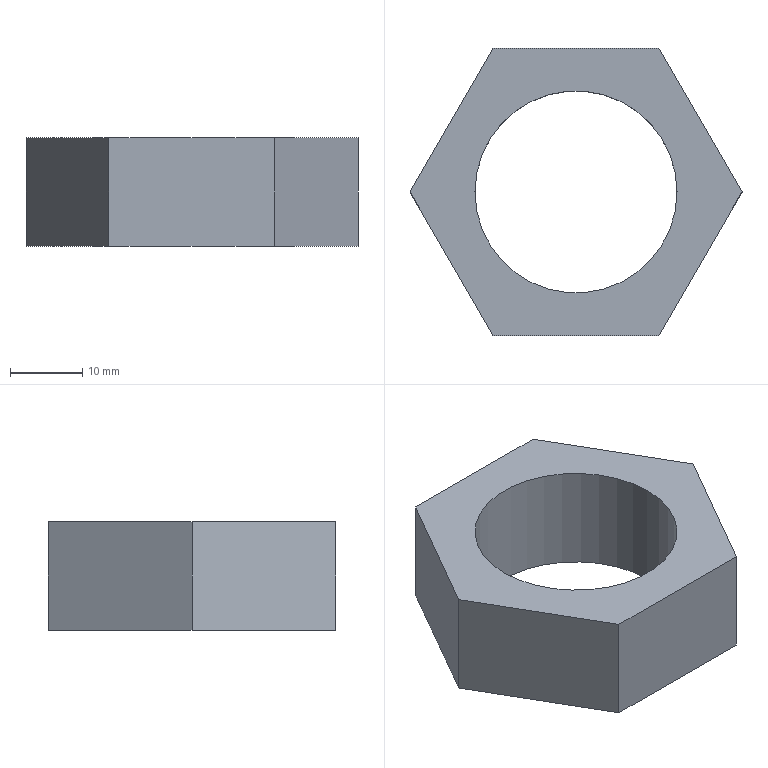Part | NX | features solid 2 | 1 solid | 9 faces | box 46 x 39.837 x 15 mm | volume 11379 mm3 | plane 8 | cylinder 1 | commonest cylinder face diameters 28 x1
STEP:
#1=CARTESIAN_POINT('',(11.5,-174.919,-70.));
#2=VERTEX_POINT('',#1);
#3=CARTESIAN_POINT('',(-11.5,-174.919,-70.));
#4=VERTEX_POINT('',#3);
#5=CARTESIAN_POINT('',(11.5,-174.919,-70.));
#6=DIRECTION('',(-1.,0.,0.));
#7=VECTOR('',#6,1000.);
#8=LINE('',#5,#7);
#9=EDGE_CURVE('',#2,#4,#8,.T.);
#10=ORIENTED_EDGE('',*,*,#9,.F.);
#11=CARTESIAN_POINT('',(11.5,-174.919,-55.));
#12=VERTEX_POINT('',#11);
#13=CARTESIAN_POINT('',(11.5,-174.919,-55.));
#14=DIRECTION('',(0.,0.,-1.));
#15=VECTOR('',#14,1000.);
#16=LINE('',#13,#15);
#17=EDGE_CURVE('',#12,#2,#16,.T.);
#18=ORIENTED_EDGE('',*,*,#17,.F.);
#19=CARTESIAN_POINT('',(-11.5,-174.919,-55.));
#20=VERTEX_POINT('',#19);
#21=CARTESIAN_POINT('',(11.5,-174.919,-55.));
#22=DIRECTION('',(-1.,0.,0.));
#23=VECTOR('',#22,1000.);
#24=LINE('',#21,#23);
#25=EDGE_CURVE('',#12,#20,#24,.T.);
#26=ORIENTED_EDGE('',*,*,#25,.T.);
#27=CARTESIAN_POINT('',(-11.5,-174.919,-55.));
#28=DIRECTION('',(0.,0.,-1.));
#29=VECTOR('',#28,1000.);
#30=LINE('',#27,#29);
#31=EDGE_CURVE('',#20,#4,#30,.T.);
#32=ORIENTED_EDGE('',*,*,#31,.T.);
#33=EDGE_LOOP('',(#10,#18,#26,#32));
#34=FACE_BOUND('',#33,.T.);
#35=CARTESIAN_POINT('',(11.5,-174.919,-55.));
#36=DIRECTION('',(0.,-1.,0.));
#37=DIRECTION('',(0.,0.,-1.));
#38=AXIS2_PLACEMENT_3D('',#35,#36,#37);
#39=PLANE('',#38);
#40=ADVANCED_FACE('',(#34),#39,.T.);
#41=CARTESIAN_POINT('',(-23.,-155.,-70.));
#42=VERTEX_POINT('',#41);
#43=CARTESIAN_POINT('',(-11.5,-174.919,-70.));
#44=DIRECTION('',(-0.5,0.866,0.));
#45=VECTOR('',#44,1000.);
#46=LINE('',#43,#45);
#47=EDGE_CURVE('',#4,#42,#46,.T.);
#48=ORIENTED_EDGE('',*,*,#47,.F.);
#49=ORIENTED_EDGE('',*,*,#31,.F.);
#50=CARTESIAN_POINT('',(-23.,-155.,-55.));
#51=VERTEX_POINT('',#50);
#52=CARTESIAN_POINT('',(-11.5,-174.919,-55.));
#53=DIRECTION('',(-0.5,0.866,0.));
#54=VECTOR('',#53,1000.);
#55=LINE('',#52,#54);
#56=EDGE_CURVE('',#20,#51,#55,.T.);
#57=ORIENTED_EDGE('',*,*,#56,.T.);
#58=CARTESIAN_POINT('',(-23.,-155.,-55.));
#59=DIRECTION('',(0.,0.,-1.));
#60=VECTOR('',#59,1000.);
#61=LINE('',#58,#60);
#62=EDGE_CURVE('',#51,#42,#61,.T.);
#63=ORIENTED_EDGE('',*,*,#62,.T.);
#64=EDGE_LOOP('',(#48,#49,#57,#63));
#65=FACE_BOUND('',#64,.T.);
#66=CARTESIAN_POINT('',(-11.5,-174.919,-55.));
#67=DIRECTION('',(-0.866,-0.5,0.));
#68=DIRECTION('',(0.5,-0.866,0.));
#69=AXIS2_PLACEMENT_3D('',#66,#67,#68);
#70=PLANE('',#69);
#71=ADVANCED_FACE('',(#65),#70,.T.);
#72=CARTESIAN_POINT('',(-11.5,-135.081,-70.));
#73=VERTEX_POINT('',#72);
#74=CARTESIAN_POINT('',(-23.,-155.,-70.));
#75=DIRECTION('',(0.5,0.866,0.));
#76=VECTOR('',#75,1000.);
#77=LINE('',#74,#76);
#78=EDGE_CURVE('',#42,#73,#77,.T.);
#79=ORIENTED_EDGE('',*,*,#78,.F.);
#80=ORIENTED_EDGE('',*,*,#62,.F.);
#81=CARTESIAN_POINT('',(-11.5,-135.081,-55.));
#82=VERTEX_POINT('',#81);
#83=CARTESIAN_POINT('',(-23.,-155.,-55.));
#84=DIRECTION('',(0.5,0.866,0.));
#85=VECTOR('',#84,1000.);
#86=LINE('',#83,#85);
#87=EDGE_CURVE('',#51,#82,#86,.T.);
#88=ORIENTED_EDGE('',*,*,#87,.T.);
#89=CARTESIAN_POINT('',(-11.5,-135.081,-55.));
#90=DIRECTION('',(0.,0.,-1.));
#91=VECTOR('',#90,1000.);
#92=LINE('',#89,#91);
#93=EDGE_CURVE('',#82,#73,#92,.T.);
#94=ORIENTED_EDGE('',*,*,#93,.T.);
#95=EDGE_LOOP('',(#79,#80,#88,#94));
#96=FACE_BOUND('',#95,.T.);
#97=CARTESIAN_POINT('',(-23.,-155.,-55.));
#98=DIRECTION('',(-0.866,0.5,0.));
#99=DIRECTION('',(-0.5,-0.866,0.));
#100=AXIS2_PLACEMENT_3D('',#97,#98,#99);
#101=PLANE('',#100);
#102=ADVANCED_FACE('',(#96),#101,.T.);
#103=CARTESIAN_POINT('',(11.5,-135.081,-70.));
#104=VERTEX_POINT('',#103);
#105=CARTESIAN_POINT('',(-11.5,-135.081,-70.));
#106=DIRECTION('',(1.,0.,0.));
#107=VECTOR('',#106,1000.);
#108=LINE('',#105,#107);
#109=EDGE_CURVE('',#73,#104,#108,.T.);
#110=ORIENTED_EDGE('',*,*,#109,.F.);
#111=ORIENTED_EDGE('',*,*,#93,.F.);
#112=CARTESIAN_POINT('',(11.5,-135.081,-55.));
#113=VERTEX_POINT('',#112);
#114=CARTESIAN_POINT('',(-11.5,-135.081,-55.));
#115=DIRECTION('',(1.,0.,0.));
#116=VECTOR('',#115,1000.);
#117=LINE('',#114,#116);
#118=EDGE_CURVE('',#82,#113,#117,.T.);
#119=ORIENTED_EDGE('',*,*,#118,.T.);
#120=CARTESIAN_POINT('',(11.5,-135.081,-55.));
#121=DIRECTION('',(0.,0.,-1.));
#122=VECTOR('',#121,1000.);
#123=LINE('',#120,#122);
#124=EDGE_CURVE('',#113,#104,#123,.T.);
#125=ORIENTED_EDGE('',*,*,#124,.T.);
#126=EDGE_LOOP('',(#110,#111,#119,#125));
#127=FACE_BOUND('',#126,.T.);
#128=CARTESIAN_POINT('',(-11.5,-135.081,-55.));
#129=DIRECTION('',(0.,1.,0.));
#130=DIRECTION('',(0.,0.,1.));
#131=AXIS2_PLACEMENT_3D('',#128,#129,#130);
#132=PLANE('',#131);
#133=ADVANCED_FACE('',(#127),#132,.T.);
#134=CARTESIAN_POINT('',(23.,-155.,-70.));
#135=VERTEX_POINT('',#134);
#136=CARTESIAN_POINT('',(11.5,-135.081,-70.));
#137=DIRECTION('',(0.5,-0.866,0.));
#138=VECTOR('',#137,1000.);
#139=LINE('',#136,#138);
#140=EDGE_CURVE('',#104,#135,#139,.T.);
#141=ORIENTED_EDGE('',*,*,#140,.F.);
#142=ORIENTED_EDGE('',*,*,#124,.F.);
#143=CARTESIAN_POINT('',(23.,-155.,-55.));
#144=VERTEX_POINT('',#143);
#145=CARTESIAN_POINT('',(11.5,-135.081,-55.));
#146=DIRECTION('',(0.5,-0.866,0.));
#147=VECTOR('',#146,1000.);
#148=LINE('',#145,#147);
#149=EDGE_CURVE('',#113,#144,#148,.T.);
#150=ORIENTED_EDGE('',*,*,#149,.T.);
#151=CARTESIAN_POINT('',(23.,-155.,-55.));
#152=DIRECTION('',(0.,0.,-1.));
#153=VECTOR('',#152,1000.);
#154=LINE('',#151,#153);
#155=EDGE_CURVE('',#144,#135,#154,.T.);
#156=ORIENTED_EDGE('',*,*,#155,.T.);
#157=EDGE_LOOP('',(#141,#142,#150,#156));
#158=FACE_BOUND('',#157,.T.);
#159=CARTESIAN_POINT('',(11.5,-135.081,-55.));
#160=DIRECTION('',(0.866,0.5,0.));
#161=DIRECTION('',(-0.5,0.866,0.));
#162=AXIS2_PLACEMENT_3D('',#159,#160,#161);
#163=PLANE('',#162);
#164=ADVANCED_FACE('',(#158),#163,.T.);
#165=CARTESIAN_POINT('',(23.,-155.,-70.));
#166=DIRECTION('',(-0.5,-0.866,0.));
#167=VECTOR('',#166,1000.);
#168=LINE('',#165,#167);
#169=EDGE_CURVE('',#135,#2,#168,.T.);
#170=ORIENTED_EDGE('',*,*,#169,.F.);
#171=ORIENTED_EDGE('',*,*,#155,.F.);
#172=CARTESIAN_POINT('',(23.,-155.,-55.));
#173=DIRECTION('',(-0.5,-0.866,0.));
#174=VECTOR('',#173,1000.);
#175=LINE('',#172,#174);
#176=EDGE_CURVE('',#144,#12,#175,.T.);
#177=ORIENTED_EDGE('',*,*,#176,.T.);
#178=ORIENTED_EDGE('',*,*,#17,.T.);
#179=EDGE_LOOP('',(#170,#171,#177,#178));
#180=FACE_BOUND('',#179,.T.);
#181=CARTESIAN_POINT('',(23.,-155.,-55.));
#182=DIRECTION('',(0.866,-0.5,0.));
#183=DIRECTION('',(0.5,0.866,0.));
#184=AXIS2_PLACEMENT_3D('',#181,#182,#183);
#185=PLANE('',#184);
#186=ADVANCED_FACE('',(#180),#185,.T.);
#187=CARTESIAN_POINT('',(14.,-155.,-55.));
#188=VERTEX_POINT('',#187);
#189=CARTESIAN_POINT('',(0.,-155.,-55.));
#190=DIRECTION('',(0.,0.,1.));
#191=DIRECTION('',(1.,0.,0.));
#192=AXIS2_PLACEMENT_3D('',#189,#190,#191);
#193=CIRCLE('',#192,14.);
#194=EDGE_CURVE('',#188,#188,#193,.T.);
#195=ORIENTED_EDGE('',*,*,#194,.T.);
#196=EDGE_LOOP('',(#195));
#197=FACE_BOUND('',#196,.T.);
#198=CARTESIAN_POINT('',(14.,-155.,-70.));
#199=VERTEX_POINT('',#198);
#200=CARTESIAN_POINT('',(0.,-155.,-70.));
#201=DIRECTION('',(0.,0.,1.));
#202=DIRECTION('',(1.,0.,0.));
#203=AXIS2_PLACEMENT_3D('',#200,#201,#202);
#204=CIRCLE('',#203,14.);
#205=EDGE_CURVE('',#199,#199,#204,.T.);
#206=ORIENTED_EDGE('',*,*,#205,.F.);
#207=EDGE_LOOP('',(#206));
#208=FACE_BOUND('',#207,.T.);
#209=CARTESIAN_POINT('',(0.,-155.,-55.));
#210=DIRECTION('',(0.,0.,-1.));
#211=DIRECTION('',(-1.,0.,0.));
#212=AXIS2_PLACEMENT_3D('',#209,#210,#211);
#213=CYLINDRICAL_SURFACE('',#212,14.);
#214=ADVANCED_FACE('',(#197,#208),#213,.F.);
#215=ORIENTED_EDGE('',*,*,#25,.F.);
#216=ORIENTED_EDGE('',*,*,#176,.F.);
#217=ORIENTED_EDGE('',*,*,#149,.F.);
#218=ORIENTED_EDGE('',*,*,#118,.F.);
#219=ORIENTED_EDGE('',*,*,#87,.F.);
#220=ORIENTED_EDGE('',*,*,#56,.F.);
#221=EDGE_LOOP('',(#215,#216,#217,#218,#219,#220));
#222=FACE_BOUND('',#221,.T.);
#223=ORIENTED_EDGE('',*,*,#194,.F.);
#224=EDGE_LOOP('',(#223));
#225=FACE_BOUND('',#224,.T.);
#226=CARTESIAN_POINT('',(-11.5,-174.919,-55.));
#227=DIRECTION('',(0.,0.,-1.));
#228=DIRECTION('',(-1.,0.,0.));
#229=AXIS2_PLACEMENT_3D('',#226,#227,#228);
#230=PLANE('',#229);
#231=ADVANCED_FACE('',(#222,#225),#230,.F.);
#232=ORIENTED_EDGE('',*,*,#9,.T.);
#233=ORIENTED_EDGE('',*,*,#47,.T.);
#234=ORIENTED_EDGE('',*,*,#78,.T.);
#235=ORIENTED_EDGE('',*,*,#109,.T.);
#236=ORIENTED_EDGE('',*,*,#140,.T.);
#237=ORIENTED_EDGE('',*,*,#169,.T.);
#238=EDGE_LOOP('',(#232,#233,#234,#235,#236,#237));
#239=FACE_BOUND('',#238,.T.);
#240=ORIENTED_EDGE('',*,*,#205,.T.);
#241=EDGE_LOOP('',(#240));
#242=FACE_BOUND('',#241,.T.);
#243=CARTESIAN_POINT('',(-11.5,-174.919,-70.));
#244=DIRECTION('',(0.,0.,-1.));
#245=DIRECTION('',(-1.,0.,0.));
#246=AXIS2_PLACEMENT_3D('',#243,#244,#245);
#247=PLANE('',#246);
#248=ADVANCED_FACE('',(#239,#242),#247,.T.);
#249=CLOSED_SHELL('',(#40,#71,#102,#133,#164,#186,#214,#231,#248));
#250=MANIFOLD_SOLID_BREP('',#249);
#251=(LENGTH_UNIT()NAMED_UNIT(*)SI_UNIT(.MILLI.,.METRE.));
#252=UNCERTAINTY_MEASURE_WITH_UNIT(LENGTH_MEASURE(0.00001),#251,'','');
#253=(NAMED_UNIT(*)PLANE_ANGLE_UNIT()SI_UNIT($,.RADIAN.));
#254=(NAMED_UNIT(*)SI_UNIT($,.STERADIAN.)SOLID_ANGLE_UNIT());
#255=(GEOMETRIC_REPRESENTATION_CONTEXT(3)GLOBAL_UNCERTAINTY_ASSIGNED_CONTEXT((#252))GLOBAL_UNIT_ASSIGNED_CONTEXT((#251,#253,#254))REPRESENTATION_CONTEXT('',''));
#256=ADVANCED_BREP_SHAPE_REPRESENTATION('',(#250),#255);